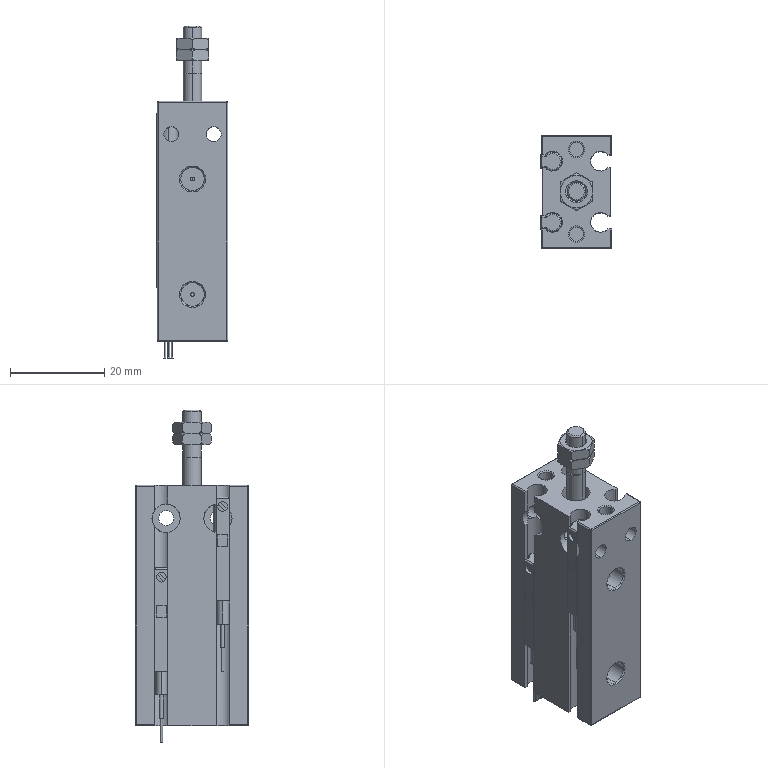Part | NX | 5 solids | 293 faces | box 15.21 x 24 x 70.5 mm | volume 13834 mm3 | cylinder 136 | plane 103 | torus 22 | cone 20 | sphere 8 | spline 4 | commonest cylinder face diameters 0.5 x28 3.2 x16 4 x14 6 x14 0.75 x12 4.2 x12